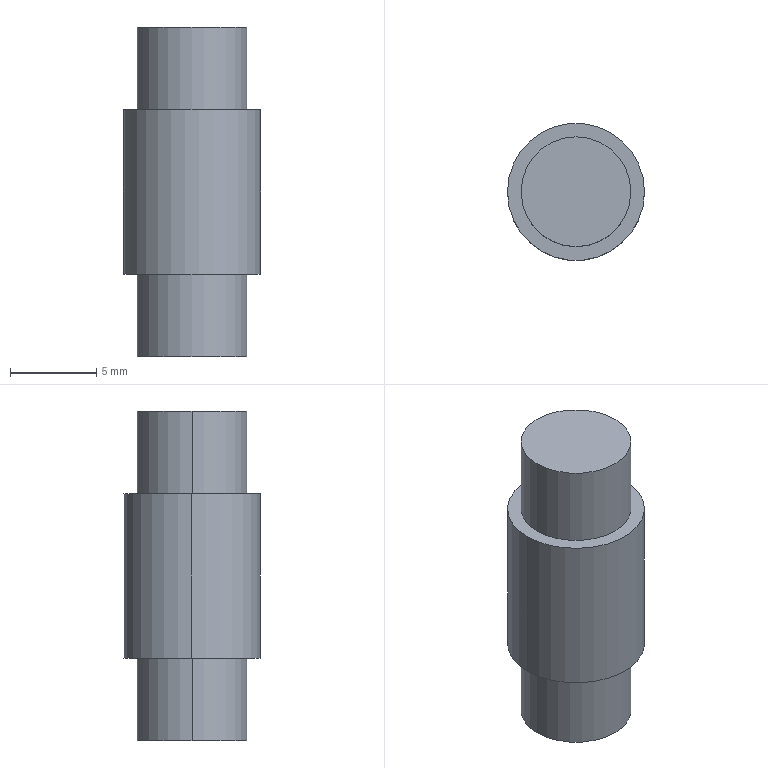Part | SolidWorks | features Extrusion 1, ICE 1 | 1 solid | 10 faces | box 7.925 x 7.925 x 19.05 mm | volume 771.469 mm3 | cylinder 6 | plane 4 | commonest cylinder face diameters 6.35 x4 7.925 x2
STEP:
#1=CARTESIAN_POINT('',(3.175,0.,-9.525));
#2=VERTEX_POINT('',#1);
#3=CARTESIAN_POINT('',(-3.175,0.,-9.525));
#4=VERTEX_POINT('',#3);
#5=CARTESIAN_POINT('',(0.,0.,-9.525));
#6=DIRECTION('',(0.,0.,1.));
#7=DIRECTION('',(1.,0.,0.));
#8=AXIS2_PLACEMENT_3D('',#5,#6,#7);
#9=CIRCLE('',#8,3.175);
#10=EDGE_CURVE('',#2,#4,#9,.T.);
#11=ORIENTED_EDGE('',*,*,#10,.T.);
#12=CARTESIAN_POINT('',(-3.175,0.,-4.763));
#13=VERTEX_POINT('',#12);
#14=CARTESIAN_POINT('',(-3.175,0.,-9.525));
#15=DIRECTION('',(0.,0.,1.));
#16=VECTOR('',#15,1000.);
#17=LINE('',#14,#16);
#18=EDGE_CURVE('',#4,#13,#17,.T.);
#19=ORIENTED_EDGE('',*,*,#18,.T.);
#20=CARTESIAN_POINT('',(3.175,0.,-4.763));
#21=VERTEX_POINT('',#20);
#22=CARTESIAN_POINT('',(0.,0.,-4.763));
#23=DIRECTION('',(0.,0.,1.));
#24=DIRECTION('',(1.,0.,0.));
#25=AXIS2_PLACEMENT_3D('',#22,#23,#24);
#26=CIRCLE('',#25,3.175);
#27=EDGE_CURVE('',#21,#13,#26,.T.);
#28=ORIENTED_EDGE('',*,*,#27,.F.);
#29=CARTESIAN_POINT('',(3.175,0.,-9.525));
#30=DIRECTION('',(0.,0.,1.));
#31=VECTOR('',#30,1000.);
#32=LINE('',#29,#31);
#33=EDGE_CURVE('',#2,#21,#32,.T.);
#34=ORIENTED_EDGE('',*,*,#33,.F.);
#35=EDGE_LOOP('',(#11,#19,#28,#34));
#36=FACE_OUTER_BOUND('',#35,.T.);
#37=CARTESIAN_POINT('',(0.,0.,-9.525));
#38=DIRECTION('',(0.,0.,1.));
#39=DIRECTION('',(1.,0.,0.));
#40=AXIS2_PLACEMENT_3D('',#37,#38,#39);
#41=CYLINDRICAL_SURFACE('',#40,3.175);
#42=ADVANCED_FACE('',(#36),#41,.T.);
#43=CARTESIAN_POINT('',(3.175,0.,4.763));
#44=VERTEX_POINT('',#43);
#45=CARTESIAN_POINT('',(-3.175,0.,4.763));
#46=VERTEX_POINT('',#45);
#47=CARTESIAN_POINT('',(0.,0.,4.763));
#48=DIRECTION('',(0.,0.,1.));
#49=DIRECTION('',(1.,0.,0.));
#50=AXIS2_PLACEMENT_3D('',#47,#48,#49);
#51=CIRCLE('',#50,3.175);
#52=EDGE_CURVE('',#44,#46,#51,.T.);
#53=ORIENTED_EDGE('',*,*,#52,.T.);
#54=CARTESIAN_POINT('',(-3.175,0.,9.525));
#55=VERTEX_POINT('',#54);
#56=CARTESIAN_POINT('',(-3.175,0.,-9.525));
#57=DIRECTION('',(0.,0.,1.));
#58=VECTOR('',#57,1000.);
#59=LINE('',#56,#58);
#60=EDGE_CURVE('',#46,#55,#59,.T.);
#61=ORIENTED_EDGE('',*,*,#60,.T.);
#62=CARTESIAN_POINT('',(3.175,0.,9.525));
#63=VERTEX_POINT('',#62);
#64=CARTESIAN_POINT('',(0.,0.,9.525));
#65=DIRECTION('',(0.,0.,1.));
#66=DIRECTION('',(1.,0.,0.));
#67=AXIS2_PLACEMENT_3D('',#64,#65,#66);
#68=CIRCLE('',#67,3.175);
#69=EDGE_CURVE('',#63,#55,#68,.T.);
#70=ORIENTED_EDGE('',*,*,#69,.F.);
#71=CARTESIAN_POINT('',(3.175,0.,-9.525));
#72=DIRECTION('',(0.,0.,1.));
#73=VECTOR('',#72,1000.);
#74=LINE('',#71,#73);
#75=EDGE_CURVE('',#44,#63,#74,.T.);
#76=ORIENTED_EDGE('',*,*,#75,.F.);
#77=EDGE_LOOP('',(#53,#61,#70,#76));
#78=FACE_OUTER_BOUND('',#77,.T.);
#79=CARTESIAN_POINT('',(0.,0.,-9.525));
#80=DIRECTION('',(0.,0.,1.));
#81=DIRECTION('',(1.,0.,0.));
#82=AXIS2_PLACEMENT_3D('',#79,#80,#81);
#83=CYLINDRICAL_SURFACE('',#82,3.175);
#84=ADVANCED_FACE('',(#78),#83,.T.);
#85=CARTESIAN_POINT('',(3.962,0.,-4.763));
#86=VERTEX_POINT('',#85);
#87=CARTESIAN_POINT('',(-3.962,0.,-4.763));
#88=VERTEX_POINT('',#87);
#89=CARTESIAN_POINT('',(0.,0.,-4.763));
#90=DIRECTION('',(0.,0.,1.));
#91=DIRECTION('',(1.,0.,0.));
#92=AXIS2_PLACEMENT_3D('',#89,#90,#91);
#93=CIRCLE('',#92,3.962);
#94=EDGE_CURVE('',#86,#88,#93,.T.);
#95=ORIENTED_EDGE('',*,*,#94,.T.);
#96=CARTESIAN_POINT('',(-3.962,0.,4.763));
#97=VERTEX_POINT('',#96);
#98=CARTESIAN_POINT('',(-3.962,0.,-4.763));
#99=DIRECTION('',(0.,0.,1.));
#100=VECTOR('',#99,1000.);
#101=LINE('',#98,#100);
#102=EDGE_CURVE('',#88,#97,#101,.T.);
#103=ORIENTED_EDGE('',*,*,#102,.T.);
#104=CARTESIAN_POINT('',(3.962,0.,4.763));
#105=VERTEX_POINT('',#104);
#106=CARTESIAN_POINT('',(0.,0.,4.763));
#107=DIRECTION('',(0.,0.,1.));
#108=DIRECTION('',(1.,0.,0.));
#109=AXIS2_PLACEMENT_3D('',#106,#107,#108);
#110=CIRCLE('',#109,3.962);
#111=EDGE_CURVE('',#105,#97,#110,.T.);
#112=ORIENTED_EDGE('',*,*,#111,.F.);
#113=CARTESIAN_POINT('',(3.962,0.,-4.763));
#114=DIRECTION('',(0.,0.,1.));
#115=VECTOR('',#114,1000.);
#116=LINE('',#113,#115);
#117=EDGE_CURVE('',#86,#105,#116,.T.);
#118=ORIENTED_EDGE('',*,*,#117,.F.);
#119=EDGE_LOOP('',(#95,#103,#112,#118));
#120=FACE_OUTER_BOUND('',#119,.T.);
#121=CARTESIAN_POINT('',(0.,0.,-4.763));
#122=DIRECTION('',(0.,0.,1.));
#123=DIRECTION('',(1.,0.,0.));
#124=AXIS2_PLACEMENT_3D('',#121,#122,#123);
#125=CYLINDRICAL_SURFACE('',#124,3.962);
#126=ADVANCED_FACE('',(#120),#125,.T.);
#127=ORIENTED_EDGE('',*,*,#102,.F.);
#128=CARTESIAN_POINT('',(0.,0.,-4.763));
#129=DIRECTION('',(0.,0.,1.));
#130=DIRECTION('',(1.,0.,0.));
#131=AXIS2_PLACEMENT_3D('',#128,#129,#130);
#132=CIRCLE('',#131,3.962);
#133=EDGE_CURVE('',#88,#86,#132,.T.);
#134=ORIENTED_EDGE('',*,*,#133,.T.);
#135=ORIENTED_EDGE('',*,*,#117,.T.);
#136=CARTESIAN_POINT('',(0.,0.,4.763));
#137=DIRECTION('',(0.,0.,1.));
#138=DIRECTION('',(1.,0.,0.));
#139=AXIS2_PLACEMENT_3D('',#136,#137,#138);
#140=CIRCLE('',#139,3.962);
#141=EDGE_CURVE('',#97,#105,#140,.T.);
#142=ORIENTED_EDGE('',*,*,#141,.F.);
#143=EDGE_LOOP('',(#127,#134,#135,#142));
#144=FACE_OUTER_BOUND('',#143,.T.);
#145=CARTESIAN_POINT('',(0.,0.,-4.763));
#146=DIRECTION('',(0.,0.,1.));
#147=DIRECTION('',(1.,0.,0.));
#148=AXIS2_PLACEMENT_3D('',#145,#146,#147);
#149=CYLINDRICAL_SURFACE('',#148,3.962);
#150=ADVANCED_FACE('',(#144),#149,.T.);
#151=ORIENTED_EDGE('',*,*,#27,.T.);
#152=CARTESIAN_POINT('',(0.,0.,-4.763));
#153=DIRECTION('',(0.,0.,1.));
#154=DIRECTION('',(1.,0.,0.));
#155=AXIS2_PLACEMENT_3D('',#152,#153,#154);
#156=CIRCLE('',#155,3.175);
#157=EDGE_CURVE('',#13,#21,#156,.T.);
#158=ORIENTED_EDGE('',*,*,#157,.T.);
#159=EDGE_LOOP('',(#151,#158));
#160=FACE_BOUND('',#159,.T.);
#161=ORIENTED_EDGE('',*,*,#94,.F.);
#162=ORIENTED_EDGE('',*,*,#133,.F.);
#163=EDGE_LOOP('',(#161,#162));
#164=FACE_OUTER_BOUND('',#163,.T.);
#165=CARTESIAN_POINT('',(0.,0.,-4.763));
#166=DIRECTION('',(0.,0.,1.));
#167=DIRECTION('',(1.,0.,0.));
#168=AXIS2_PLACEMENT_3D('',#165,#166,#167);
#169=PLANE('',#168);
#170=ADVANCED_FACE('',(#160,#164),#169,.F.);
#171=ORIENTED_EDGE('',*,*,#52,.F.);
#172=CARTESIAN_POINT('',(0.,0.,4.763));
#173=DIRECTION('',(0.,0.,1.));
#174=DIRECTION('',(1.,0.,0.));
#175=AXIS2_PLACEMENT_3D('',#172,#173,#174);
#176=CIRCLE('',#175,3.175);
#177=EDGE_CURVE('',#46,#44,#176,.T.);
#178=ORIENTED_EDGE('',*,*,#177,.F.);
#179=EDGE_LOOP('',(#171,#178));
#180=FACE_BOUND('',#179,.T.);
#181=ORIENTED_EDGE('',*,*,#111,.T.);
#182=ORIENTED_EDGE('',*,*,#141,.T.);
#183=EDGE_LOOP('',(#181,#182));
#184=FACE_OUTER_BOUND('',#183,.T.);
#185=CARTESIAN_POINT('',(0.,0.,4.763));
#186=DIRECTION('',(0.,0.,1.));
#187=DIRECTION('',(1.,0.,0.));
#188=AXIS2_PLACEMENT_3D('',#185,#186,#187);
#189=PLANE('',#188);
#190=ADVANCED_FACE('',(#180,#184),#189,.T.);
#191=ORIENTED_EDGE('',*,*,#69,.T.);
#192=CARTESIAN_POINT('',(0.,0.,9.525));
#193=DIRECTION('',(0.,0.,1.));
#194=DIRECTION('',(1.,0.,0.));
#195=AXIS2_PLACEMENT_3D('',#192,#193,#194);
#196=CIRCLE('',#195,3.175);
#197=EDGE_CURVE('',#55,#63,#196,.T.);
#198=ORIENTED_EDGE('',*,*,#197,.T.);
#199=EDGE_LOOP('',(#191,#198));
#200=FACE_OUTER_BOUND('',#199,.T.);
#201=CARTESIAN_POINT('',(0.,0.,9.525));
#202=DIRECTION('',(0.,0.,1.));
#203=DIRECTION('',(1.,0.,0.));
#204=AXIS2_PLACEMENT_3D('',#201,#202,#203);
#205=PLANE('',#204);
#206=ADVANCED_FACE('',(#200),#205,.T.);
#207=ORIENTED_EDGE('',*,*,#60,.F.);
#208=ORIENTED_EDGE('',*,*,#177,.T.);
#209=ORIENTED_EDGE('',*,*,#75,.T.);
#210=ORIENTED_EDGE('',*,*,#197,.F.);
#211=EDGE_LOOP('',(#207,#208,#209,#210));
#212=FACE_OUTER_BOUND('',#211,.T.);
#213=CARTESIAN_POINT('',(0.,0.,-9.525));
#214=DIRECTION('',(0.,0.,1.));
#215=DIRECTION('',(1.,0.,0.));
#216=AXIS2_PLACEMENT_3D('',#213,#214,#215);
#217=CYLINDRICAL_SURFACE('',#216,3.175);
#218=ADVANCED_FACE('',(#212),#217,.T.);
#219=ORIENTED_EDGE('',*,*,#18,.F.);
#220=CARTESIAN_POINT('',(0.,0.,-9.525));
#221=DIRECTION('',(0.,0.,1.));
#222=DIRECTION('',(1.,0.,0.));
#223=AXIS2_PLACEMENT_3D('',#220,#221,#222);
#224=CIRCLE('',#223,3.175);
#225=EDGE_CURVE('',#4,#2,#224,.T.);
#226=ORIENTED_EDGE('',*,*,#225,.T.);
#227=ORIENTED_EDGE('',*,*,#33,.T.);
#228=ORIENTED_EDGE('',*,*,#157,.F.);
#229=EDGE_LOOP('',(#219,#226,#227,#228));
#230=FACE_OUTER_BOUND('',#229,.T.);
#231=CARTESIAN_POINT('',(0.,0.,-9.525));
#232=DIRECTION('',(0.,0.,1.));
#233=DIRECTION('',(1.,0.,0.));
#234=AXIS2_PLACEMENT_3D('',#231,#232,#233);
#235=CYLINDRICAL_SURFACE('',#234,3.175);
#236=ADVANCED_FACE('',(#230),#235,.T.);
#237=ORIENTED_EDGE('',*,*,#10,.F.);
#238=ORIENTED_EDGE('',*,*,#225,.F.);
#239=EDGE_LOOP('',(#237,#238));
#240=FACE_OUTER_BOUND('',#239,.T.);
#241=CARTESIAN_POINT('',(0.,0.,-9.525));
#242=DIRECTION('',(0.,0.,1.));
#243=DIRECTION('',(1.,0.,0.));
#244=AXIS2_PLACEMENT_3D('',#241,#242,#243);
#245=PLANE('',#244);
#246=ADVANCED_FACE('',(#240),#245,.F.);
#247=CLOSED_SHELL('',(#42,#84,#126,#150,#170,#190,#206,#218,#236,#246));
#248=MANIFOLD_SOLID_BREP('',#247);
#249=CARTESIAN_POINT('',(0.,0.,0.));
#250=DIRECTION('',(0.,0.,1.));
#251=DIRECTION('',(1.,0.,0.));
#252=AXIS2_PLACEMENT_3D('',#249,#250,#251);
#253=(LENGTH_UNIT()NAMED_UNIT(*)SI_UNIT(.MILLI.,.METRE.));
#254=UNCERTAINTY_MEASURE_WITH_UNIT(LENGTH_MEASURE(0.00001),#253,'','');
#255=(NAMED_UNIT(*)PLANE_ANGLE_UNIT()SI_UNIT($,.RADIAN.));
#256=(NAMED_UNIT(*)SI_UNIT($,.STERADIAN.)SOLID_ANGLE_UNIT());
#257=(GEOMETRIC_REPRESENTATION_CONTEXT(3)GLOBAL_UNCERTAINTY_ASSIGNED_CONTEXT((#254))GLOBAL_UNIT_ASSIGNED_CONTEXT((#253,#255,#256))REPRESENTATION_CONTEXT('',''));
#258=ADVANCED_BREP_SHAPE_REPRESENTATION('',(#248,#252),#257);